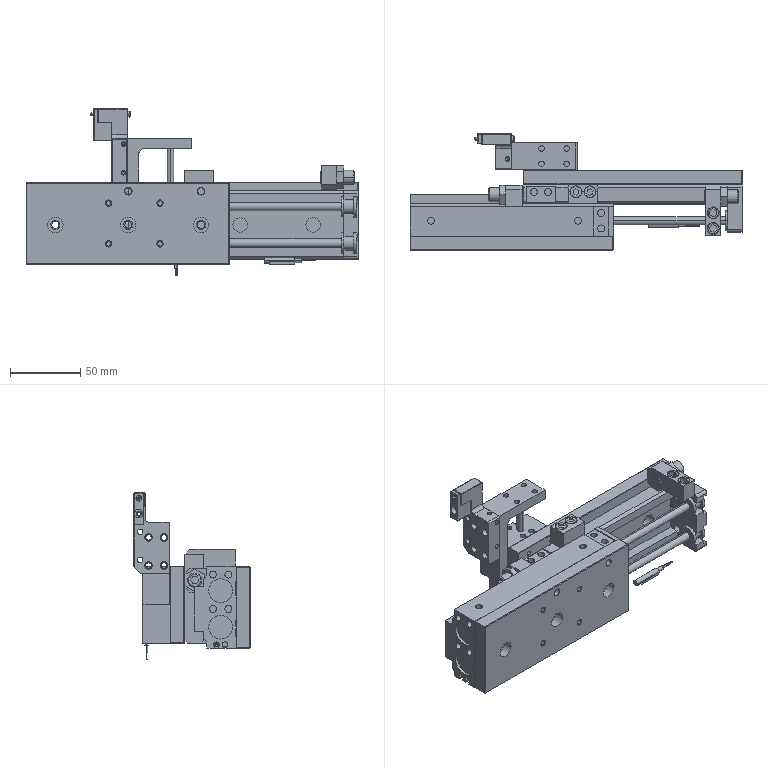Part | NX | 18 solids | 1004 faces | box 237 x 83 x 119 mm | volume 506515 mm3 | plane 504 | cylinder 406 | cone 94 | commonest cylinder face diameters 5 x93 4 x58 2.5 x38 0.5 x16 1 x16 6 x16